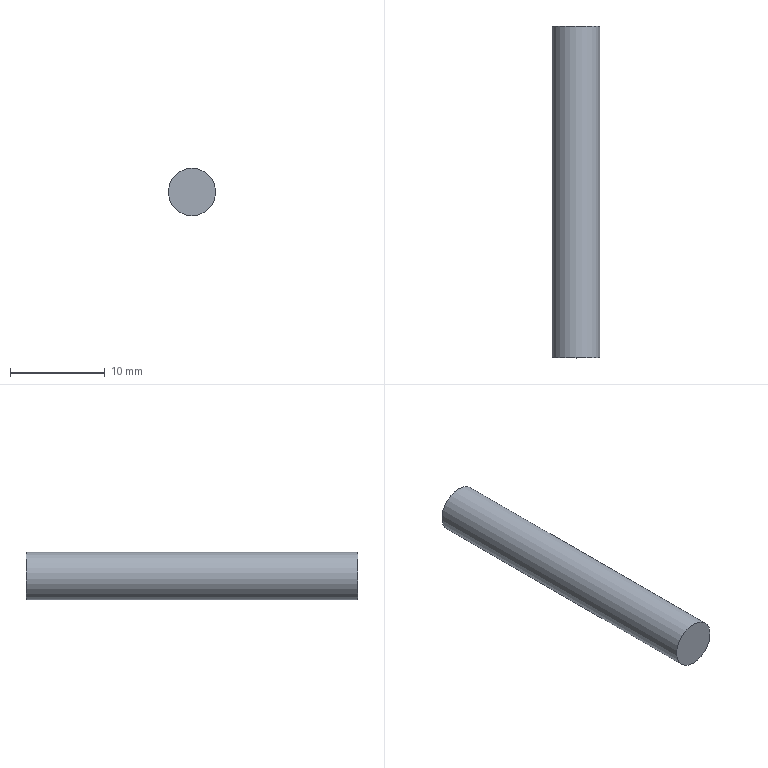Part | STEP file | solid 94 | 1 solid | 3 faces | box 5 x 35 x 5 mm | volume 687.223 mm3 | plane 2 | cylinder 1 | commonest cylinder face diameters 5 x1